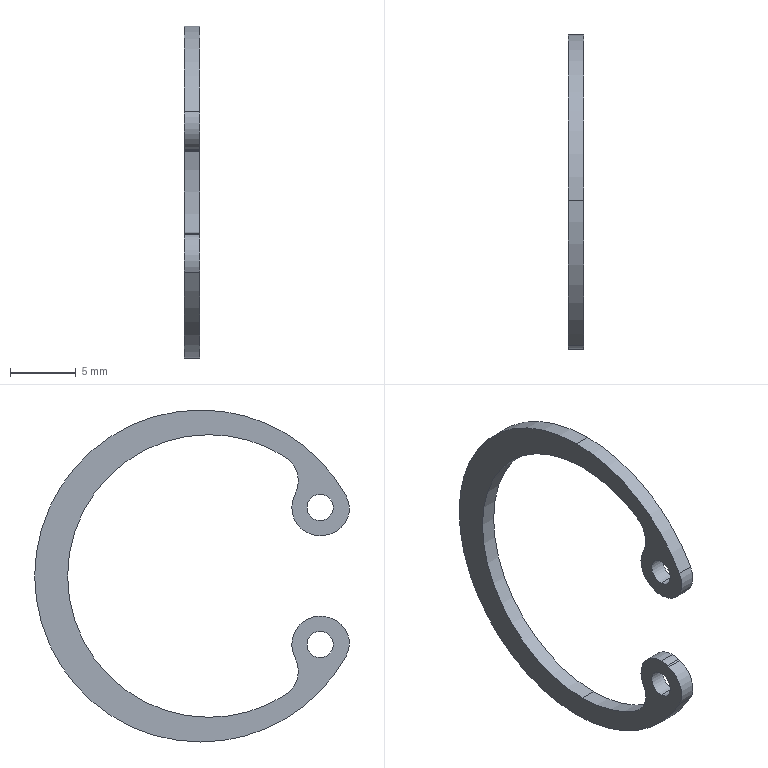Part | STEP file | MISUMI C-type retaining ring RTWN24-1 | 1 solid | 21 faces | box 1.2 x 23.885 x 25.2 mm | volume 171.114 mm3 | cylinder 17 | plane 4 | commonest cylinder face diameters 4.3 x5 2 x4 21.45 x3 25.2 x3 4 x2
STEP:
#1=CARTESIAN_POINT('',(0.6,-9.064,6.2));
#2=VERTEX_POINT('',#1);
#3=CARTESIAN_POINT('',(0.6,-9.064,4.2));
#4=VERTEX_POINT('',#3);
#5=CARTESIAN_POINT('',(0.6,-9.064,5.2));
#6=DIRECTION('',(1.,0.,0.));
#7=DIRECTION('',(0.,0.,-1.));
#8=AXIS2_PLACEMENT_3D('',#5,#6,#7);
#9=CIRCLE('',#8,1.);
#10=EDGE_CURVE('',#2,#4,#9,.T.);
#11=ORIENTED_EDGE('',*,*,#10,.T.);
#12=CARTESIAN_POINT('',(-0.6,-9.064,4.2));
#13=VERTEX_POINT('',#12);
#14=CARTESIAN_POINT('',(0.6,-9.064,4.2));
#15=DIRECTION('',(-1.,0.,0.));
#16=VECTOR('',#15,1000.);
#17=LINE('',#14,#16);
#18=EDGE_CURVE('',#4,#13,#17,.T.);
#19=ORIENTED_EDGE('',*,*,#18,.T.);
#20=CARTESIAN_POINT('',(-0.6,-9.064,6.2));
#21=VERTEX_POINT('',#20);
#22=CARTESIAN_POINT('',(-0.6,-9.064,5.2));
#23=DIRECTION('',(1.,0.,0.));
#24=DIRECTION('',(0.,0.,-1.));
#25=AXIS2_PLACEMENT_3D('',#22,#23,#24);
#26=CIRCLE('',#25,1.);
#27=EDGE_CURVE('',#21,#13,#26,.T.);
#28=ORIENTED_EDGE('',*,*,#27,.F.);
#29=CARTESIAN_POINT('',(0.6,-9.064,6.2));
#30=DIRECTION('',(-1.,0.,0.));
#31=VECTOR('',#30,1000.);
#32=LINE('',#29,#31);
#33=EDGE_CURVE('',#2,#21,#32,.T.);
#34=ORIENTED_EDGE('',*,*,#33,.F.);
#35=EDGE_LOOP('',(#11,#19,#28,#34));
#36=FACE_OUTER_BOUND('',#35,.T.);
#37=CARTESIAN_POINT('',(0.6,-9.064,5.2));
#38=DIRECTION('',(-1.,0.,0.));
#39=DIRECTION('',(0.,0.,1.));
#40=AXIS2_PLACEMENT_3D('',#37,#38,#39);
#41=CYLINDRICAL_SURFACE('',#40,1.);
#42=ADVANCED_FACE('',(#36),#41,.F.);
#43=CARTESIAN_POINT('',(0.6,-9.064,-4.2));
#44=VERTEX_POINT('',#43);
#45=CARTESIAN_POINT('',(0.6,-9.064,-6.2));
#46=VERTEX_POINT('',#45);
#47=CARTESIAN_POINT('',(0.6,-9.064,-5.2));
#48=DIRECTION('',(1.,0.,0.));
#49=DIRECTION('',(0.,0.,-1.));
#50=AXIS2_PLACEMENT_3D('',#47,#48,#49);
#51=CIRCLE('',#50,1.);
#52=EDGE_CURVE('',#44,#46,#51,.T.);
#53=ORIENTED_EDGE('',*,*,#52,.T.);
#54=CARTESIAN_POINT('',(-0.6,-9.064,-6.2));
#55=VERTEX_POINT('',#54);
#56=CARTESIAN_POINT('',(0.6,-9.064,-6.2));
#57=DIRECTION('',(-1.,0.,0.));
#58=VECTOR('',#57,1000.);
#59=LINE('',#56,#58);
#60=EDGE_CURVE('',#46,#55,#59,.T.);
#61=ORIENTED_EDGE('',*,*,#60,.T.);
#62=CARTESIAN_POINT('',(-0.6,-9.064,-4.2));
#63=VERTEX_POINT('',#62);
#64=CARTESIAN_POINT('',(-0.6,-9.064,-5.2));
#65=DIRECTION('',(1.,0.,0.));
#66=DIRECTION('',(0.,0.,-1.));
#67=AXIS2_PLACEMENT_3D('',#64,#65,#66);
#68=CIRCLE('',#67,1.);
#69=EDGE_CURVE('',#63,#55,#68,.T.);
#70=ORIENTED_EDGE('',*,*,#69,.F.);
#71=CARTESIAN_POINT('',(0.6,-9.064,-4.2));
#72=DIRECTION('',(-1.,0.,0.));
#73=VECTOR('',#72,1000.);
#74=LINE('',#71,#73);
#75=EDGE_CURVE('',#44,#63,#74,.T.);
#76=ORIENTED_EDGE('',*,*,#75,.F.);
#77=EDGE_LOOP('',(#53,#61,#70,#76));
#78=FACE_OUTER_BOUND('',#77,.T.);
#79=CARTESIAN_POINT('',(0.6,-9.064,-5.2));
#80=DIRECTION('',(-1.,0.,0.));
#81=DIRECTION('',(0.,0.,1.));
#82=AXIS2_PLACEMENT_3D('',#79,#80,#81);
#83=CYLINDRICAL_SURFACE('',#82,1.);
#84=ADVANCED_FACE('',(#78),#83,.F.);
#85=CARTESIAN_POINT('',(0.6,-9.064,-3.05));
#86=VERTEX_POINT('',#85);
#87=CARTESIAN_POINT('',(0.6,-9.728,-3.155));
#88=VERTEX_POINT('',#87);
#89=CARTESIAN_POINT('',(0.6,-9.064,-5.2));
#90=DIRECTION('',(1.,0.,0.));
#91=DIRECTION('',(0.,0.,-1.));
#92=AXIS2_PLACEMENT_3D('',#89,#90,#91);
#93=CIRCLE('',#92,2.15);
#94=EDGE_CURVE('',#86,#88,#93,.T.);
#95=ORIENTED_EDGE('',*,*,#94,.F.);
#96=CARTESIAN_POINT('',(-0.6,-9.064,-3.05));
#97=VERTEX_POINT('',#96);
#98=CARTESIAN_POINT('',(0.6,-9.064,-3.05));
#99=DIRECTION('',(-1.,0.,0.));
#100=VECTOR('',#99,1000.);
#101=LINE('',#98,#100);
#102=EDGE_CURVE('',#86,#97,#101,.T.);
#103=ORIENTED_EDGE('',*,*,#102,.T.);
#104=CARTESIAN_POINT('',(-0.6,-9.728,-3.155));
#105=VERTEX_POINT('',#104);
#106=CARTESIAN_POINT('',(-0.6,-9.064,-5.2));
#107=DIRECTION('',(1.,0.,0.));
#108=DIRECTION('',(0.,0.,-1.));
#109=AXIS2_PLACEMENT_3D('',#106,#107,#108);
#110=CIRCLE('',#109,2.15);
#111=EDGE_CURVE('',#97,#105,#110,.T.);
#112=ORIENTED_EDGE('',*,*,#111,.T.);
#113=CARTESIAN_POINT('',(0.6,-9.728,-3.155));
#114=DIRECTION('',(-1.,0.,0.));
#115=VECTOR('',#114,1000.);
#116=LINE('',#113,#115);
#117=EDGE_CURVE('',#88,#105,#116,.T.);
#118=ORIENTED_EDGE('',*,*,#117,.F.);
#119=EDGE_LOOP('',(#95,#103,#112,#118));
#120=FACE_OUTER_BOUND('',#119,.T.);
#121=CARTESIAN_POINT('',(0.6,-9.064,-5.2));
#122=DIRECTION('',(-1.,0.,0.));
#123=DIRECTION('',(0.,0.,1.));
#124=AXIS2_PLACEMENT_3D('',#121,#122,#123);
#125=CYLINDRICAL_SURFACE('',#124,2.15);
#126=ADVANCED_FACE('',(#120),#125,.T.);
#127=CARTESIAN_POINT('',(0.6,-0.625,-10.725));
#128=VERTEX_POINT('',#127);
#129=CARTESIAN_POINT('',(0.6,-6.427,-9.02));
#130=VERTEX_POINT('',#129);
#131=CARTESIAN_POINT('',(0.6,-0.625,0.));
#132=DIRECTION('',(-1.,0.,0.));
#133=DIRECTION('',(0.,0.,1.));
#134=AXIS2_PLACEMENT_3D('',#131,#132,#133);
#135=CIRCLE('',#134,10.725);
#136=EDGE_CURVE('',#128,#130,#135,.T.);
#137=ORIENTED_EDGE('',*,*,#136,.F.);
#138=CARTESIAN_POINT('',(-0.6,-0.625,-10.725));
#139=VERTEX_POINT('',#138);
#140=CARTESIAN_POINT('',(0.6,-0.625,-10.725));
#141=DIRECTION('',(-1.,0.,0.));
#142=VECTOR('',#141,1000.);
#143=LINE('',#140,#142);
#144=EDGE_CURVE('',#128,#139,#143,.T.);
#145=ORIENTED_EDGE('',*,*,#144,.T.);
#146=CARTESIAN_POINT('',(-0.6,-6.427,-9.02));
#147=VERTEX_POINT('',#146);
#148=CARTESIAN_POINT('',(-0.6,-0.625,0.));
#149=DIRECTION('',(-1.,0.,0.));
#150=DIRECTION('',(0.,0.,1.));
#151=AXIS2_PLACEMENT_3D('',#148,#149,#150);
#152=CIRCLE('',#151,10.725);
#153=EDGE_CURVE('',#139,#147,#152,.T.);
#154=ORIENTED_EDGE('',*,*,#153,.T.);
#155=CARTESIAN_POINT('',(0.6,-6.427,-9.02));
#156=DIRECTION('',(-1.,0.,0.));
#157=VECTOR('',#156,1000.);
#158=LINE('',#155,#157);
#159=EDGE_CURVE('',#130,#147,#158,.T.);
#160=ORIENTED_EDGE('',*,*,#159,.F.);
#161=EDGE_LOOP('',(#137,#145,#154,#160));
#162=FACE_OUTER_BOUND('',#161,.T.);
#163=CARTESIAN_POINT('',(0.6,-0.625,0.));
#164=DIRECTION('',(-1.,0.,0.));
#165=DIRECTION('',(0.,0.,1.));
#166=AXIS2_PLACEMENT_3D('',#163,#164,#165);
#167=CYLINDRICAL_SURFACE('',#166,10.725);
#168=ADVANCED_FACE('',(#162),#167,.F.);
#169=ORIENTED_EDGE('',*,*,#144,.F.);
#170=CARTESIAN_POINT('',(0.6,-0.625,10.725));
#171=VERTEX_POINT('',#170);
#172=CARTESIAN_POINT('',(0.6,-0.625,0.));
#173=DIRECTION('',(-1.,0.,0.));
#174=DIRECTION('',(0.,0.,1.));
#175=AXIS2_PLACEMENT_3D('',#172,#173,#174);
#176=CIRCLE('',#175,10.725);
#177=EDGE_CURVE('',#171,#128,#176,.T.);
#178=ORIENTED_EDGE('',*,*,#177,.F.);
#179=CARTESIAN_POINT('',(-0.6,-0.625,10.725));
#180=VERTEX_POINT('',#179);
#181=CARTESIAN_POINT('',(0.6,-0.625,10.725));
#182=DIRECTION('',(-1.,0.,0.));
#183=VECTOR('',#182,1000.);
#184=LINE('',#181,#183);
#185=EDGE_CURVE('',#171,#180,#184,.T.);
#186=ORIENTED_EDGE('',*,*,#185,.T.);
#187=CARTESIAN_POINT('',(-0.6,-0.625,0.));
#188=DIRECTION('',(-1.,0.,0.));
#189=DIRECTION('',(0.,0.,1.));
#190=AXIS2_PLACEMENT_3D('',#187,#188,#189);
#191=CIRCLE('',#190,10.725);
#192=EDGE_CURVE('',#180,#139,#191,.T.);
#193=ORIENTED_EDGE('',*,*,#192,.T.);
#194=EDGE_LOOP('',(#169,#178,#186,#193));
#195=FACE_OUTER_BOUND('',#194,.T.);
#196=CARTESIAN_POINT('',(0.6,-0.625,0.));
#197=DIRECTION('',(-1.,0.,0.));
#198=DIRECTION('',(0.,0.,1.));
#199=AXIS2_PLACEMENT_3D('',#196,#197,#198);
#200=CYLINDRICAL_SURFACE('',#199,10.725);
#201=ADVANCED_FACE('',(#195),#200,.F.);
#202=CARTESIAN_POINT('',(0.6,0.,-12.6));
#203=VERTEX_POINT('',#202);
#204=CARTESIAN_POINT('',(0.6,0.,12.6));
#205=VERTEX_POINT('',#204);
#206=CARTESIAN_POINT('',(0.6,0.,0.));
#207=DIRECTION('',(1.,0.,0.));
#208=DIRECTION('',(0.,0.,-1.));
#209=AXIS2_PLACEMENT_3D('',#206,#207,#208);
#210=CIRCLE('',#209,12.6);
#211=EDGE_CURVE('',#203,#205,#210,.T.);
#212=ORIENTED_EDGE('',*,*,#211,.F.);
#213=CARTESIAN_POINT('',(-0.6,0.,-12.6));
#214=VERTEX_POINT('',#213);
#215=CARTESIAN_POINT('',(0.6,0.,-12.6));
#216=DIRECTION('',(-1.,0.,0.));
#217=VECTOR('',#216,1000.);
#218=LINE('',#215,#217);
#219=EDGE_CURVE('',#203,#214,#218,.T.);
#220=ORIENTED_EDGE('',*,*,#219,.T.);
#221=CARTESIAN_POINT('',(-0.6,0.,12.6));
#222=VERTEX_POINT('',#221);
#223=CARTESIAN_POINT('',(-0.6,0.,0.));
#224=DIRECTION('',(1.,0.,0.));
#225=DIRECTION('',(0.,0.,-1.));
#226=AXIS2_PLACEMENT_3D('',#223,#224,#225);
#227=CIRCLE('',#226,12.6);
#228=EDGE_CURVE('',#214,#222,#227,.T.);
#229=ORIENTED_EDGE('',*,*,#228,.T.);
#230=CARTESIAN_POINT('',(0.6,0.,12.6));
#231=DIRECTION('',(-1.,0.,0.));
#232=VECTOR('',#231,1000.);
#233=LINE('',#230,#232);
#234=EDGE_CURVE('',#205,#222,#233,.T.);
#235=ORIENTED_EDGE('',*,*,#234,.F.);
#236=EDGE_LOOP('',(#212,#220,#229,#235));
#237=FACE_OUTER_BOUND('',#236,.T.);
#238=CARTESIAN_POINT('',(0.6,0.,0.));
#239=DIRECTION('',(-1.,0.,0.));
#240=DIRECTION('',(0.,0.,1.));
#241=AXIS2_PLACEMENT_3D('',#238,#239,#240);
#242=CYLINDRICAL_SURFACE('',#241,12.6);
#243=ADVANCED_FACE('',(#237),#242,.T.);
#244=CARTESIAN_POINT('',(0.6,-11.037,6.079));
#245=VERTEX_POINT('',#244);
#246=CARTESIAN_POINT('',(0.6,0.,0.));
#247=DIRECTION('',(1.,0.,0.));
#248=DIRECTION('',(0.,0.,-1.));
#249=AXIS2_PLACEMENT_3D('',#246,#247,#248);
#250=CIRCLE('',#249,12.6);
#251=EDGE_CURVE('',#205,#245,#250,.T.);
#252=ORIENTED_EDGE('',*,*,#251,.F.);
#253=ORIENTED_EDGE('',*,*,#234,.T.);
#254=CARTESIAN_POINT('',(-0.6,-11.037,6.079));
#255=VERTEX_POINT('',#254);
#256=CARTESIAN_POINT('',(-0.6,0.,0.));
#257=DIRECTION('',(1.,0.,0.));
#258=DIRECTION('',(0.,0.,-1.));
#259=AXIS2_PLACEMENT_3D('',#256,#257,#258);
#260=CIRCLE('',#259,12.6);
#261=EDGE_CURVE('',#222,#255,#260,.T.);
#262=ORIENTED_EDGE('',*,*,#261,.T.);
#263=CARTESIAN_POINT('',(0.6,-11.037,6.079));
#264=DIRECTION('',(-1.,0.,0.));
#265=VECTOR('',#264,1000.);
#266=LINE('',#263,#265);
#267=EDGE_CURVE('',#245,#255,#266,.T.);
#268=ORIENTED_EDGE('',*,*,#267,.F.);
#269=EDGE_LOOP('',(#252,#253,#262,#268));
#270=FACE_OUTER_BOUND('',#269,.T.);
#271=CARTESIAN_POINT('',(0.6,0.,0.));
#272=DIRECTION('',(-1.,0.,0.));
#273=DIRECTION('',(0.,0.,1.));
#274=AXIS2_PLACEMENT_3D('',#271,#272,#273);
#275=CYLINDRICAL_SURFACE('',#274,12.6);
#276=ADVANCED_FACE('',(#270),#275,.T.);
#277=ORIENTED_EDGE('',*,*,#52,.F.);
#278=CARTESIAN_POINT('',(0.6,-9.064,-5.2));
#279=DIRECTION('',(1.,0.,0.));
#280=DIRECTION('',(0.,0.,-1.));
#281=AXIS2_PLACEMENT_3D('',#278,#279,#280);
#282=CIRCLE('',#281,1.);
#283=EDGE_CURVE('',#46,#44,#282,.T.);
#284=ORIENTED_EDGE('',*,*,#283,.F.);
#285=EDGE_LOOP('',(#277,#284));
#286=FACE_BOUND('',#285,.T.);
#287=CARTESIAN_POINT('',(0.6,-9.902,-3.211));
#288=VERTEX_POINT('',#287);
#289=CARTESIAN_POINT('',(0.6,-11.037,-6.079));
#290=VERTEX_POINT('',#289);
#291=CARTESIAN_POINT('',(0.6,-9.285,-5.114));
#292=DIRECTION('',(1.,0.,0.));
#293=DIRECTION('',(0.,0.,-1.));
#294=AXIS2_PLACEMENT_3D('',#291,#292,#293);
#295=CIRCLE('',#294,2.);
#296=EDGE_CURVE('',#288,#290,#295,.T.);
#297=ORIENTED_EDGE('',*,*,#296,.T.);
#298=CARTESIAN_POINT('',(0.6,0.,0.));
#299=DIRECTION('',(1.,0.,0.));
#300=DIRECTION('',(0.,0.,-1.));
#301=AXIS2_PLACEMENT_3D('',#298,#299,#300);
#302=CIRCLE('',#301,12.6);
#303=EDGE_CURVE('',#290,#203,#302,.T.);
#304=ORIENTED_EDGE('',*,*,#303,.T.);
#305=ORIENTED_EDGE('',*,*,#211,.T.);
#306=ORIENTED_EDGE('',*,*,#251,.T.);
#307=CARTESIAN_POINT('',(0.6,-9.902,3.211));
#308=VERTEX_POINT('',#307);
#309=CARTESIAN_POINT('',(0.6,-9.285,5.114));
#310=DIRECTION('',(1.,0.,0.));
#311=DIRECTION('',(0.,0.,-1.));
#312=AXIS2_PLACEMENT_3D('',#309,#310,#311);
#313=CIRCLE('',#312,2.);
#314=EDGE_CURVE('',#245,#308,#313,.T.);
#315=ORIENTED_EDGE('',*,*,#314,.T.);
#316=CARTESIAN_POINT('',(0.6,-9.728,3.155));
#317=VERTEX_POINT('',#316);
#318=CARTESIAN_POINT('',(0.6,-9.902,3.211));
#319=DIRECTION('',(0.,0.9512,-0.3085));
#320=VECTOR('',#319,1000.);
#321=LINE('',#318,#320);
#322=EDGE_CURVE('',#308,#317,#321,.T.);
#323=ORIENTED_EDGE('',*,*,#322,.T.);
#324=CARTESIAN_POINT('',(0.6,-7.164,6.206));
#325=VERTEX_POINT('',#324);
#326=CARTESIAN_POINT('',(0.6,-9.064,5.2));
#327=DIRECTION('',(1.,0.,0.));
#328=DIRECTION('',(0.,0.,-1.));
#329=AXIS2_PLACEMENT_3D('',#326,#327,#328);
#330=CIRCLE('',#329,2.15);
#331=EDGE_CURVE('',#317,#325,#330,.T.);
#332=ORIENTED_EDGE('',*,*,#331,.T.);
#333=CARTESIAN_POINT('',(0.6,-6.427,9.02));
#334=VERTEX_POINT('',#333);
#335=CARTESIAN_POINT('',(0.6,-5.264,7.212));
#336=DIRECTION('',(-1.,0.,0.));
#337=DIRECTION('',(0.,0.,1.));
#338=AXIS2_PLACEMENT_3D('',#335,#336,#337);
#339=CIRCLE('',#338,2.15);
#340=EDGE_CURVE('',#325,#334,#339,.T.);
#341=ORIENTED_EDGE('',*,*,#340,.T.);
#342=CARTESIAN_POINT('',(0.6,-0.625,0.));
#343=DIRECTION('',(-1.,0.,0.));
#344=DIRECTION('',(0.,0.,1.));
#345=AXIS2_PLACEMENT_3D('',#342,#343,#344);
#346=CIRCLE('',#345,10.725);
#347=EDGE_CURVE('',#334,#171,#346,.T.);
#348=ORIENTED_EDGE('',*,*,#347,.T.);
#349=ORIENTED_EDGE('',*,*,#177,.T.);
#350=ORIENTED_EDGE('',*,*,#136,.T.);
#351=CARTESIAN_POINT('',(0.6,-7.164,-6.206));
#352=VERTEX_POINT('',#351);
#353=CARTESIAN_POINT('',(0.6,-5.264,-7.212));
#354=DIRECTION('',(-1.,0.,0.));
#355=DIRECTION('',(0.,0.,1.));
#356=AXIS2_PLACEMENT_3D('',#353,#354,#355);
#357=CIRCLE('',#356,2.15);
#358=EDGE_CURVE('',#130,#352,#357,.T.);
#359=ORIENTED_EDGE('',*,*,#358,.T.);
#360=CARTESIAN_POINT('',(0.6,-9.064,-5.2));
#361=DIRECTION('',(1.,0.,0.));
#362=DIRECTION('',(0.,0.,-1.));
#363=AXIS2_PLACEMENT_3D('',#360,#361,#362);
#364=CIRCLE('',#363,2.15);
#365=EDGE_CURVE('',#352,#86,#364,.T.);
#366=ORIENTED_EDGE('',*,*,#365,.T.);
#367=ORIENTED_EDGE('',*,*,#94,.T.);
#368=CARTESIAN_POINT('',(0.6,-9.728,-3.155));
#369=DIRECTION('',(0.,-0.9512,-0.3085));
#370=VECTOR('',#369,1000.);
#371=LINE('',#368,#370);
#372=EDGE_CURVE('',#88,#288,#371,.T.);
#373=ORIENTED_EDGE('',*,*,#372,.T.);
#374=EDGE_LOOP('',(#297,#304,#305,#306,#315,#323,#332,#341,#348,#349,#350,#359,#366,#367,#373));
#375=FACE_OUTER_BOUND('',#374,.T.);
#376=ORIENTED_EDGE('',*,*,#10,.F.);
#377=CARTESIAN_POINT('',(0.6,-9.064,5.2));
#378=DIRECTION('',(1.,0.,0.));
#379=DIRECTION('',(0.,0.,-1.));
#380=AXIS2_PLACEMENT_3D('',#377,#378,#379);
#381=CIRCLE('',#380,1.);
#382=EDGE_CURVE('',#4,#2,#381,.T.);
#383=ORIENTED_EDGE('',*,*,#382,.F.);
#384=EDGE_LOOP('',(#376,#383));
#385=FACE_BOUND('',#384,.T.);
#386=CARTESIAN_POINT('',(0.6,-9.285,-5.114));
#387=DIRECTION('',(1.,0.,0.));
#388=DIRECTION('',(0.,0.,-1.));
#389=AXIS2_PLACEMENT_3D('',#386,#387,#388);
#390=PLANE('',#389);
#391=ADVANCED_FACE('',(#286,#375,#385),#390,.T.);
#392=CARTESIAN_POINT('',(-0.6,-9.902,-3.211));
#393=VERTEX_POINT('',#392);
#394=CARTESIAN_POINT('',(0.6,-9.902,-3.211));
#395=DIRECTION('',(-1.,0.,0.));
#396=VECTOR('',#395,1000.);
#397=LINE('',#394,#396);
#398=EDGE_CURVE('',#288,#393,#397,.T.);
#399=ORIENTED_EDGE('',*,*,#398,.T.);
#400=CARTESIAN_POINT('',(-0.6,-11.037,-6.079));
#401=VERTEX_POINT('',#400);
#402=CARTESIAN_POINT('',(-0.6,-9.285,-5.114));
#403=DIRECTION('',(1.,0.,0.));
#404=DIRECTION('',(0.,0.,-1.));
#405=AXIS2_PLACEMENT_3D('',#402,#403,#404);
#406=CIRCLE('',#405,2.);
#407=EDGE_CURVE('',#393,#401,#406,.T.);
#408=ORIENTED_EDGE('',*,*,#407,.T.);
#409=CARTESIAN_POINT('',(0.6,-11.037,-6.079));
#410=DIRECTION('',(-1.,0.,0.));
#411=VECTOR('',#410,1000.);
#412=LINE('',#409,#411);
#413=EDGE_CURVE('',#290,#401,#412,.T.);
#414=ORIENTED_EDGE('',*,*,#413,.F.);
#415=ORIENTED_EDGE('',*,*,#296,.F.);
#416=EDGE_LOOP('',(#399,#408,#414,#415));
#417=FACE_OUTER_BOUND('',#416,.T.);
#418=CARTESIAN_POINT('',(0.6,-9.285,-5.114));
#419=DIRECTION('',(-1.,0.,0.));
#420=DIRECTION('',(0.,0.,1.));
#421=AXIS2_PLACEMENT_3D('',#418,#419,#420);
#422=CYLINDRICAL_SURFACE('',#421,2.);
#423=ADVANCED_FACE('',(#417),#422,.T.);
#424=ORIENTED_EDGE('',*,*,#219,.F.);
#425=ORIENTED_EDGE('',*,*,#303,.F.);
#426=ORIENTED_EDGE('',*,*,#413,.T.);
#427=CARTESIAN_POINT('',(-0.6,0.,0.));
#428=DIRECTION('',(1.,0.,0.));
#429=DIRECTION('',(0.,0.,-1.));
#430=AXIS2_PLACEMENT_3D('',#427,#428,#429);
#431=CIRCLE('',#430,12.6);
#432=EDGE_CURVE('',#401,#214,#431,.T.);
#433=ORIENTED_EDGE('',*,*,#432,.T.);
#434=EDGE_LOOP('',(#424,#425,#426,#433));
#435=FACE_OUTER_BOUND('',#434,.T.);
#436=CARTESIAN_POINT('',(0.6,0.,0.));
#437=DIRECTION('',(-1.,0.,0.));
#438=DIRECTION('',(0.,0.,1.));
#439=AXIS2_PLACEMENT_3D('',#436,#437,#438);
#440=CYLINDRICAL_SURFACE('',#439,12.6);
#441=ADVANCED_FACE('',(#435),#440,.T.);
#442=ORIENTED_EDGE('',*,*,#267,.T.);
#443=CARTESIAN_POINT('',(-0.6,-9.902,3.211));
#444=VERTEX_POINT('',#443);
#445=CARTESIAN_POINT('',(-0.6,-9.285,5.114));
#446=DIRECTION('',(1.,0.,0.));
#447=DIRECTION('',(0.,0.,-1.));
#448=AXIS2_PLACEMENT_3D('',#445,#446,#447);
#449=CIRCLE('',#448,2.);
#450=EDGE_CURVE('',#255,#444,#449,.T.);
#451=ORIENTED_EDGE('',*,*,#450,.T.);
#452=CARTESIAN_POINT('',(0.6,-9.902,3.211));
#453=DIRECTION('',(-1.,0.,0.));
#454=VECTOR('',#453,1000.);
#455=LINE('',#452,#454);
#456=EDGE_CURVE('',#308,#444,#455,.T.);
#457=ORIENTED_EDGE('',*,*,#456,.F.);
#458=ORIENTED_EDGE('',*,*,#314,.F.);
#459=EDGE_LOOP('',(#442,#451,#457,#458));
#460=FACE_OUTER_BOUND('',#459,.T.);
#461=CARTESIAN_POINT('',(0.6,-9.285,5.114));
#462=DIRECTION('',(-1.,0.,0.));
#463=DIRECTION('',(0.,0.,1.));
#464=AXIS2_PLACEMENT_3D('',#461,#462,#463);
#465=CYLINDRICAL_SURFACE('',#464,2.);
#466=ADVANCED_FACE('',(#460),#465,.T.);
#467=ORIENTED_EDGE('',*,*,#456,.T.);
#468=CARTESIAN_POINT('',(-0.6,-9.728,3.155));
#469=VERTEX_POINT('',#468);
#470=CARTESIAN_POINT('',(-0.6,-9.902,3.211));
#471=DIRECTION('',(0.,0.9512,-0.3085));
#472=VECTOR('',#471,1000.);
#473=LINE('',#470,#472);
#474=EDGE_CURVE('',#444,#469,#473,.T.);
#475=ORIENTED_EDGE('',*,*,#474,.T.);
#476=CARTESIAN_POINT('',(0.6,-9.728,3.155));
#477=DIRECTION('',(-1.,0.,0.));
#478=VECTOR('',#477,1000.);
#479=LINE('',#476,#478);
#480=EDGE_CURVE('',#317,#469,#479,.T.);
#481=ORIENTED_EDGE('',*,*,#480,.F.);
#482=ORIENTED_EDGE('',*,*,#322,.F.);
#483=EDGE_LOOP('',(#467,#475,#481,#482));
#484=FACE_OUTER_BOUND('',#483,.T.);
#485=CARTESIAN_POINT('',(0.6,-9.902,3.211));
#486=DIRECTION('',(0.,0.3085,0.9512));
#487=DIRECTION('',(0.,-0.9512,0.3085));
#488=AXIS2_PLACEMENT_3D('',#485,#486,#487);
#489=PLANE('',#488);
#490=ADVANCED_FACE('',(#484),#489,.F.);
#491=ORIENTED_EDGE('',*,*,#480,.T.);
#492=CARTESIAN_POINT('',(-0.6,-7.164,6.206));
#493=VERTEX_POINT('',#492);
#494=CARTESIAN_POINT('',(-0.6,-9.064,5.2));
#495=DIRECTION('',(1.,0.,0.));
#496=DIRECTION('',(0.,0.,-1.));
#497=AXIS2_PLACEMENT_3D('',#494,#495,#496);
#498=CIRCLE('',#497,2.15);
#499=EDGE_CURVE('',#469,#493,#498,.T.);
#500=ORIENTED_EDGE('',*,*,#499,.T.);
#501=CARTESIAN_POINT('',(0.6,-7.164,6.206));
#502=DIRECTION('',(-1.,0.,0.));
#503=VECTOR('',#502,1000.);
#504=LINE('',#501,#503);
#505=EDGE_CURVE('',#325,#493,#504,.T.);
#506=ORIENTED_EDGE('',*,*,#505,.F.);
#507=ORIENTED_EDGE('',*,*,#331,.F.);
#508=EDGE_LOOP('',(#491,#500,#506,#507));
#509=FACE_OUTER_BOUND('',#508,.T.);
#510=CARTESIAN_POINT('',(0.6,-9.064,5.2));
#511=DIRECTION('',(-1.,0.,0.));
#512=DIRECTION('',(0.,0.,1.));
#513=AXIS2_PLACEMENT_3D('',#510,#511,#512);
#514=CYLINDRICAL_SURFACE('',#513,2.15);
#515=ADVANCED_FACE('',(#509),#514,.T.);
#516=ORIENTED_EDGE('',*,*,#505,.T.);
#517=CARTESIAN_POINT('',(-0.6,-6.427,9.02));
#518=VERTEX_POINT('',#517);
#519=CARTESIAN_POINT('',(-0.6,-5.264,7.212));
#520=DIRECTION('',(-1.,0.,0.));
#521=DIRECTION('',(0.,0.,1.));
#522=AXIS2_PLACEMENT_3D('',#519,#520,#521);
#523=CIRCLE('',#522,2.15);
#524=EDGE_CURVE('',#493,#518,#523,.T.);
#525=ORIENTED_EDGE('',*,*,#524,.T.);
#526=CARTESIAN_POINT('',(0.6,-6.427,9.02));
#527=DIRECTION('',(-1.,0.,0.));
#528=VECTOR('',#527,1000.);
#529=LINE('',#526,#528);
#530=EDGE_CURVE('',#334,#518,#529,.T.);
#531=ORIENTED_EDGE('',*,*,#530,.F.);
#532=ORIENTED_EDGE('',*,*,#340,.F.);
#533=EDGE_LOOP('',(#516,#525,#531,#532));
#534=FACE_OUTER_BOUND('',#533,.T.);
#535=CARTESIAN_POINT('',(0.6,-5.264,7.212));
#536=DIRECTION('',(-1.,0.,0.));
#537=DIRECTION('',(0.,0.,1.));
#538=AXIS2_PLACEMENT_3D('',#535,#536,#537);
#539=CYLINDRICAL_SURFACE('',#538,2.15);
#540=ADVANCED_FACE('',(#534),#539,.F.);
#541=ORIENTED_EDGE('',*,*,#185,.F.);
#542=ORIENTED_EDGE('',*,*,#347,.F.);
#543=ORIENTED_EDGE('',*,*,#530,.T.);
#544=CARTESIAN_POINT('',(-0.6,-0.625,0.));
#545=DIRECTION('',(-1.,0.,0.));
#546=DIRECTION('',(0.,0.,1.));
#547=AXIS2_PLACEMENT_3D('',#544,#545,#546);
#548=CIRCLE('',#547,10.725);
#549=EDGE_CURVE('',#518,#180,#548,.T.);
#550=ORIENTED_EDGE('',*,*,#549,.T.);
#551=EDGE_LOOP('',(#541,#542,#543,#550));
#552=FACE_OUTER_BOUND('',#551,.T.);
#553=CARTESIAN_POINT('',(0.6,-0.625,0.));
#554=DIRECTION('',(-1.,0.,0.));
#555=DIRECTION('',(0.,0.,1.));
#556=AXIS2_PLACEMENT_3D('',#553,#554,#555);
#557=CYLINDRICAL_SURFACE('',#556,10.725);
#558=ADVANCED_FACE('',(#552),#557,.F.);
#559=ORIENTED_EDGE('',*,*,#159,.T.);
#560=CARTESIAN_POINT('',(-0.6,-7.164,-6.206));
#561=VERTEX_POINT('',#560);
#562=CARTESIAN_POINT('',(-0.6,-5.264,-7.212));
#563=DIRECTION('',(-1.,0.,0.));
#564=DIRECTION('',(0.,0.,1.));
#565=AXIS2_PLACEMENT_3D('',#562,#563,#564);
#566=CIRCLE('',#565,2.15);
#567=EDGE_CURVE('',#147,#561,#566,.T.);
#568=ORIENTED_EDGE('',*,*,#567,.T.);
#569=CARTESIAN_POINT('',(0.6,-7.164,-6.206));
#570=DIRECTION('',(-1.,0.,0.));
#571=VECTOR('',#570,1000.);
#572=LINE('',#569,#571);
#573=EDGE_CURVE('',#352,#561,#572,.T.);
#574=ORIENTED_EDGE('',*,*,#573,.F.);
#575=ORIENTED_EDGE('',*,*,#358,.F.);
#576=EDGE_LOOP('',(#559,#568,#574,#575));
#577=FACE_OUTER_BOUND('',#576,.T.);
#578=CARTESIAN_POINT('',(0.6,-5.264,-7.212));
#579=DIRECTION('',(-1.,0.,0.));
#580=DIRECTION('',(0.,0.,1.));
#581=AXIS2_PLACEMENT_3D('',#578,#579,#580);
#582=CYLINDRICAL_SURFACE('',#581,2.15);
#583=ADVANCED_FACE('',(#577),#582,.F.);
#584=ORIENTED_EDGE('',*,*,#102,.F.);
#585=ORIENTED_EDGE('',*,*,#365,.F.);
#586=ORIENTED_EDGE('',*,*,#573,.T.);
#587=CARTESIAN_POINT('',(-0.6,-9.064,-5.2));
#588=DIRECTION('',(1.,0.,0.));
#589=DIRECTION('',(0.,0.,-1.));
#590=AXIS2_PLACEMENT_3D('',#587,#588,#589);
#591=CIRCLE('',#590,2.15);
#592=EDGE_CURVE('',#561,#97,#591,.T.);
#593=ORIENTED_EDGE('',*,*,#592,.T.);
#594=EDGE_LOOP('',(#584,#585,#586,#593));
#595=FACE_OUTER_BOUND('',#594,.T.);
#596=CARTESIAN_POINT('',(0.6,-9.064,-5.2));
#597=DIRECTION('',(-1.,0.,0.));
#598=DIRECTION('',(0.,0.,1.));
#599=AXIS2_PLACEMENT_3D('',#596,#597,#598);
#600=CYLINDRICAL_SURFACE('',#599,2.15);
#601=ADVANCED_FACE('',(#595),#600,.T.);
#602=ORIENTED_EDGE('',*,*,#117,.T.);
#603=CARTESIAN_POINT('',(-0.6,-9.728,-3.155));
#604=DIRECTION('',(0.,-0.9512,-0.3085));
#605=VECTOR('',#604,1000.);
#606=LINE('',#603,#605);
#607=EDGE_CURVE('',#105,#393,#606,.T.);
#608=ORIENTED_EDGE('',*,*,#607,.T.);
#609=ORIENTED_EDGE('',*,*,#398,.F.);
#610=ORIENTED_EDGE('',*,*,#372,.F.);
#611=EDGE_LOOP('',(#602,#608,#609,#610));
#612=FACE_OUTER_BOUND('',#611,.T.);
#613=CARTESIAN_POINT('',(0.6,-9.728,-3.155));
#614=DIRECTION('',(0.,0.3085,-0.9512));
#615=DIRECTION('',(0.,0.9512,0.3085));
#616=AXIS2_PLACEMENT_3D('',#613,#614,#615);
#617=PLANE('',#616);
#618=ADVANCED_FACE('',(#612),#617,.F.);
#619=ORIENTED_EDGE('',*,*,#60,.F.);
#620=ORIENTED_EDGE('',*,*,#283,.T.);
#621=ORIENTED_EDGE('',*,*,#75,.T.);
#622=CARTESIAN_POINT('',(-0.6,-9.064,-5.2));
#623=DIRECTION('',(1.,0.,0.));
#624=DIRECTION('',(0.,0.,-1.));
#625=AXIS2_PLACEMENT_3D('',#622,#623,#624);
#626=CIRCLE('',#625,1.);
#627=EDGE_CURVE('',#55,#63,#626,.T.);
#628=ORIENTED_EDGE('',*,*,#627,.F.);
#629=EDGE_LOOP('',(#619,#620,#621,#628));
#630=FACE_OUTER_BOUND('',#629,.T.);
#631=CARTESIAN_POINT('',(0.6,-9.064,-5.2));
#632=DIRECTION('',(-1.,0.,0.));
#633=DIRECTION('',(0.,0.,1.));
#634=AXIS2_PLACEMENT_3D('',#631,#632,#633);
#635=CYLINDRICAL_SURFACE('',#634,1.);
#636=ADVANCED_FACE('',(#630),#635,.F.);
#637=ORIENTED_EDGE('',*,*,#18,.F.);
#638=ORIENTED_EDGE('',*,*,#382,.T.);
#639=ORIENTED_EDGE('',*,*,#33,.T.);
#640=CARTESIAN_POINT('',(-0.6,-9.064,5.2));
#641=DIRECTION('',(1.,0.,0.));
#642=DIRECTION('',(0.,0.,-1.));
#643=AXIS2_PLACEMENT_3D('',#640,#641,#642);
#644=CIRCLE('',#643,1.);
#645=EDGE_CURVE('',#13,#21,#644,.T.);
#646=ORIENTED_EDGE('',*,*,#645,.F.);
#647=EDGE_LOOP('',(#637,#638,#639,#646));
#648=FACE_OUTER_BOUND('',#647,.T.);
#649=CARTESIAN_POINT('',(0.6,-9.064,5.2));
#650=DIRECTION('',(-1.,0.,0.));
#651=DIRECTION('',(0.,0.,1.));
#652=AXIS2_PLACEMENT_3D('',#649,#650,#651);
#653=CYLINDRICAL_SURFACE('',#652,1.);
#654=ADVANCED_FACE('',(#648),#653,.F.);
#655=ORIENTED_EDGE('',*,*,#27,.T.);
#656=ORIENTED_EDGE('',*,*,#645,.T.);
#657=EDGE_LOOP('',(#655,#656));
#658=FACE_BOUND('',#657,.T.);
#659=ORIENTED_EDGE('',*,*,#69,.T.);
#660=ORIENTED_EDGE('',*,*,#627,.T.);
#661=EDGE_LOOP('',(#659,#660));
#662=FACE_BOUND('',#661,.T.);
#663=ORIENTED_EDGE('',*,*,#407,.F.);
#664=ORIENTED_EDGE('',*,*,#607,.F.);
#665=ORIENTED_EDGE('',*,*,#111,.F.);
#666=ORIENTED_EDGE('',*,*,#592,.F.);
#667=ORIENTED_EDGE('',*,*,#567,.F.);
#668=ORIENTED_EDGE('',*,*,#153,.F.);
#669=ORIENTED_EDGE('',*,*,#192,.F.);
#670=ORIENTED_EDGE('',*,*,#549,.F.);
#671=ORIENTED_EDGE('',*,*,#524,.F.);
#672=ORIENTED_EDGE('',*,*,#499,.F.);
#673=ORIENTED_EDGE('',*,*,#474,.F.);
#674=ORIENTED_EDGE('',*,*,#450,.F.);
#675=ORIENTED_EDGE('',*,*,#261,.F.);
#676=ORIENTED_EDGE('',*,*,#228,.F.);
#677=ORIENTED_EDGE('',*,*,#432,.F.);
#678=EDGE_LOOP('',(#663,#664,#665,#666,#667,#668,#669,#670,#671,#672,#673,#674,#675,#676,#677));
#679=FACE_OUTER_BOUND('',#678,.T.);
#680=CARTESIAN_POINT('',(-0.6,-9.285,-5.114));
#681=DIRECTION('',(1.,0.,0.));
#682=DIRECTION('',(0.,0.,-1.));
#683=AXIS2_PLACEMENT_3D('',#680,#681,#682);
#684=PLANE('',#683);
#685=ADVANCED_FACE('',(#658,#662,#679),#684,.F.);
#686=CLOSED_SHELL('',(#42,#84,#126,#168,#201,#243,#276,#391,#423,#441,#466,#490,#515,#540,#558,#583,#601,#618,#636,#654,#685));
#687=MANIFOLD_SOLID_BREP('',#686);
#688=CARTESIAN_POINT('',(0.,0.,0.));
#689=DIRECTION('',(0.,0.,1.));
#690=DIRECTION('',(1.,0.,0.));
#691=AXIS2_PLACEMENT_3D('',#688,#689,#690);
#692=(LENGTH_UNIT()NAMED_UNIT(*)SI_UNIT(.MILLI.,.METRE.));
#693=UNCERTAINTY_MEASURE_WITH_UNIT(LENGTH_MEASURE(0.00001),#692,'','');
#694=(NAMED_UNIT(*)PLANE_ANGLE_UNIT()SI_UNIT($,.RADIAN.));
#695=(NAMED_UNIT(*)SI_UNIT($,.STERADIAN.)SOLID_ANGLE_UNIT());
#696=(GEOMETRIC_REPRESENTATION_CONTEXT(3)GLOBAL_UNCERTAINTY_ASSIGNED_CONTEXT((#693))GLOBAL_UNIT_ASSIGNED_CONTEXT((#692,#694,#695))REPRESENTATION_CONTEXT('',''));
#697=ADVANCED_BREP_SHAPE_REPRESENTATION('',(#687,#691),#696);